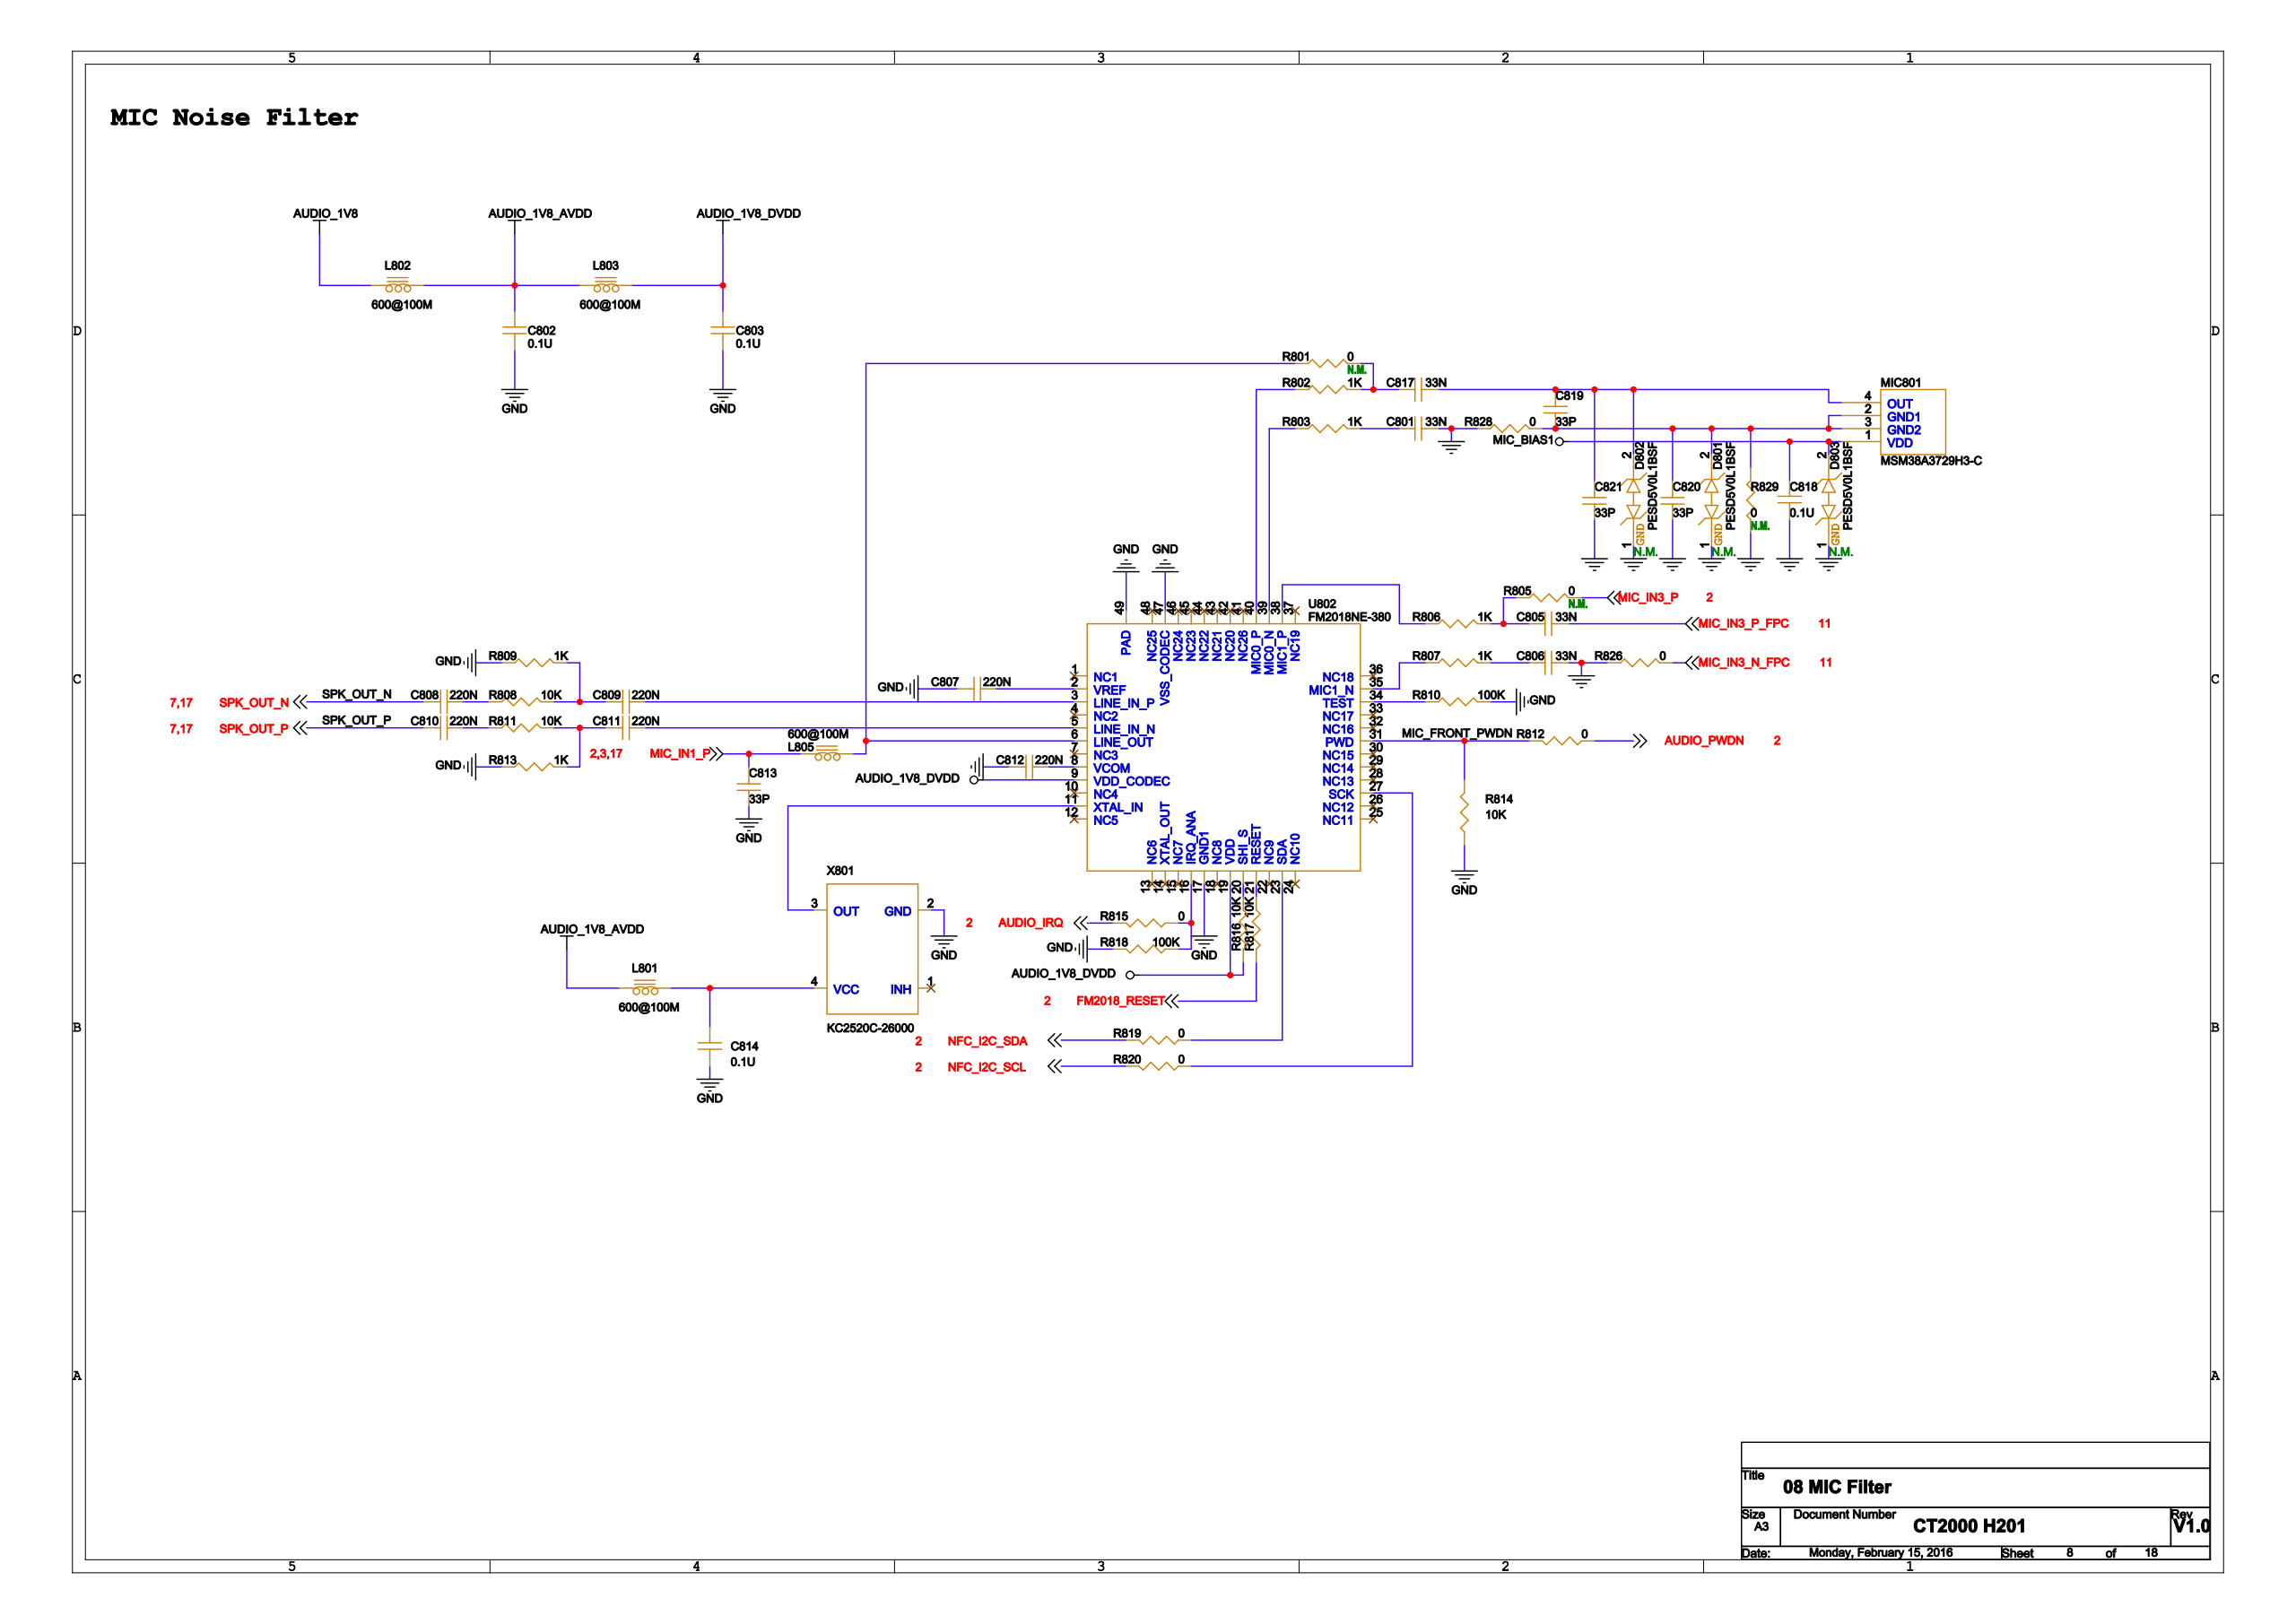Circuit board | Cadence Allegro | 573 parts | 376 nets | one sheet of the schematic
Parts on this sheet (reference | value | footprint):
C801 | 33N | C0402
C802 | 0.1U | C0402
C803 | 0.1U | C0402
C805 | 33N | C0402
C806 | 33N | C0402
C807 | 220N | C0402
C808 | 220N | C0402
C809 | 220N | C0402
C810 | 220N | C0402
C811 | 220N | C0402
C812 | 220N | C0402
C813 | 33P | C0402
C814 | 0.1U | C0402
C817 | 33N | C0402
C818 | 0.1U | C0402
C819 | 33P | C0402
C820 | 33P | C0402
C821 | 33P | C0402
D801 | PESD5V0L1BSF | DSN0603-2
D802 | PESD5V0L1BSF | DSN0603-2
D803 | PESD5V0L1BSF | DSN0603-2
L801 | 600@100M | L0402
L802 | 600@100M | L0402
L803 | 600@100M | L0402
L805 | 600@100M | L0402
MIC801 | MSM38A3729H3-C | MSM381A3729H3-C
R801 | 0 | R0402
R802 | 1K | R0402
R803 | 1K | R0402
R805 | 0 | R0402
R806 | 1K | R0402
R807 | 1K | R0402
R808 | 10K | R0402
R809 | 1K | R0402
R810 | 100K | R0402
R811 | 10K | R0402
R812 | 0 | R0402
R813 | 1K | R0402
R814 | 10K | R0402
R815 | 0 | R0402
R816 | 10K | R0402
R817 | 10K | R0402
R818 | 100K | R0402
R819 | 0 | R0402
R820 | 0 | R0402
R826 | 0 | R0402
R828 | 0 | R0402
R829 | 0 | R0402
U802 | FM2018NE-380 | FM2018NE-380
X801 | KC2520C-26000 | KC2520C
Nets of these parts (net: part-pin ...):
GND: C801-2 C802-2 C803-2 C806-2 C807-2 C812-2 C813-1 C814-2 C818-2 C820-1 C821-1 D801-1 D802-1 D803-1 R809-2 R810-2 R813-2 R814-2 R818-1 R826-2 R828-2 R829-2 X801-2 U802-17 U802-47 U802-49
MIC_IN1_P: C813-2 L805-1
MIC_IN3_P_FPC: C805-2
MIC_IN3_N_FPC: R826-1
MIC_BIAS1: C818-1 D803-2 MIC801-1
N52508514: C819-1 C820-2 D801-2 MIC801-2 MIC801-3 R828-1 R829-1
N52306772: C817-2 C819-2 C821-2 D802-2 MIC801-4
AUDIO_1V8: L802-1
FM2018_RESET: R817-2
MIC_IN3_P: R805-1
NFC_I2C_SCL: R820-2
NFC_I2C_SDA: R819-2
AUDIO_PWDN: R812-1
AUDIO_IRQ: R815-2
AUDIO_1V8_DVDD: C803-1 L803-2 R816-2 U802-9 U802-19
N46703062: C814-1 L801-2 X801-4
AUDIO_1V8_AVDD: C802-1 L801-1 L802-2 L803-1
N51972164: C801-1 R803-1
N46725522: C805-1 R805-2 R806-1
N46725514: C806-1 R807-1
N51972140: C817-1 R801-1 R802-1
N46556330: C807-1 U802-2
N46573477: C808-1 R808-1
SPK_OUT_N: C808-2
N46557507: C809-1 U802-3
N46574638: C809-2 R808-2 R809-1
N46580238: C810-1 R811-1
SPK_OUT_P: C810-2
N46581846: C811-1 U802-5
N46580240: C811-2 R811-2 R813-1
N46678998: C812-1 U802-8
N51966102: L805-2 R801-2 U802-6
MIC_FRONT_PWDN: R812-2 R814-1 U802-31
N46776965: R816-1 U802-20
N46814162: R817-1 U802-21
N46767826: R815-1 R818-2 U802-16
N46760655: R819-1 U802-23
N46751079: R820-1 U802-27
N46722843: R802-2 U802-40
N46724120: R803-2 U802-39
N46727246: R806-2 U802-38
N46729855: R807-2 U802-35
N46808776: R810-1 U802-34
N46705165: X801-3 U802-11